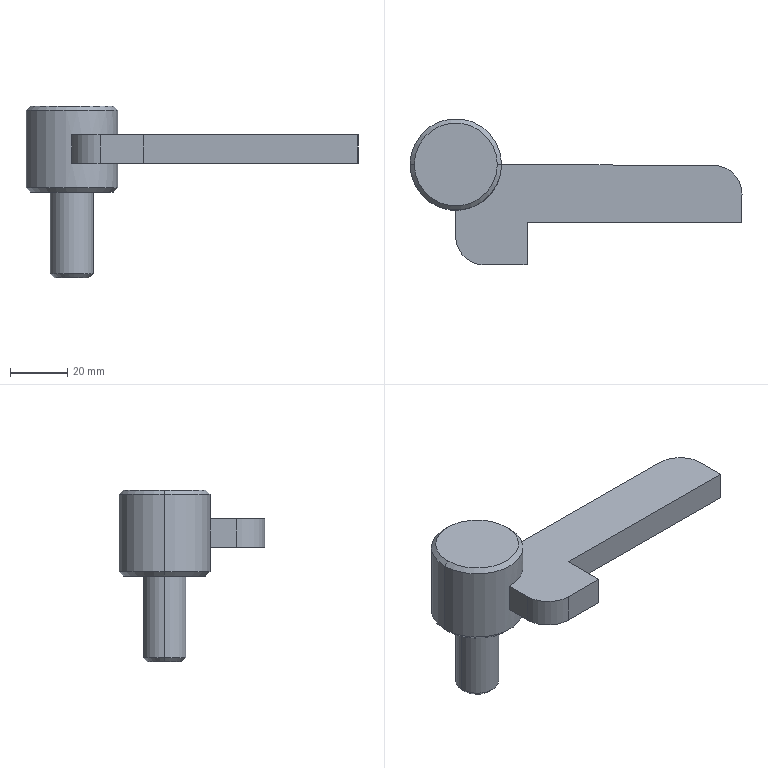Part | STEP file | Input 50 | 1 solid | 23 faces | box 115.97 x 51.074 x 60 mm | volume 50470 mm3 | plane 11 | cone 6 | cylinder 6 | commonest cylinder face diameters 15 x2 20 x2 32 x2